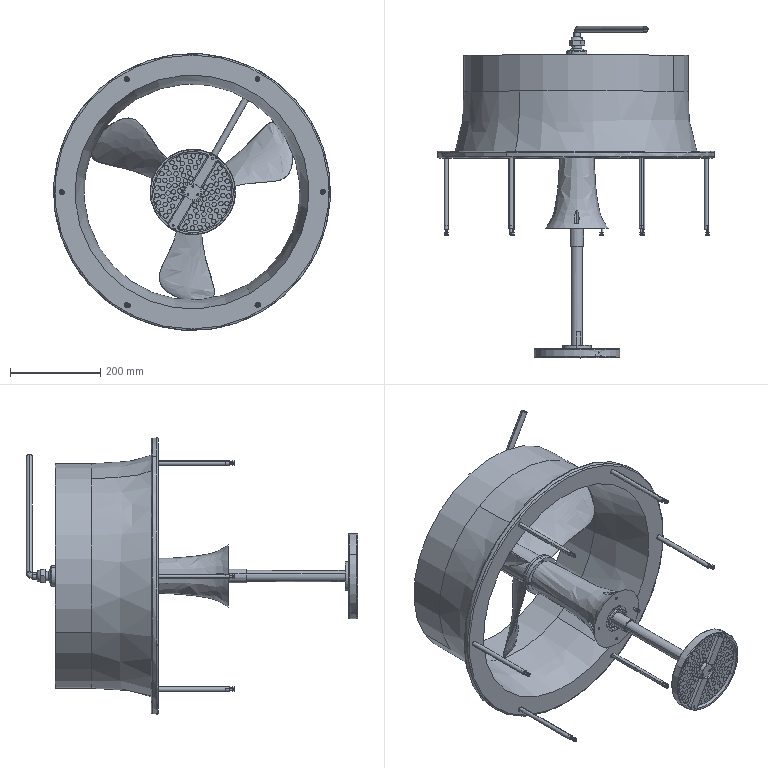Part | NX | features BREP 16 | 27 solids | 1247 faces | box 615 x 737 x 615 mm | volume 7539199 mm3 | cylinder 460 | plane 325 | torus 183 | sphere 128 | cone 80 | spline 71 | commonest cylinder face diameters 10 x201 5 x52 22 x26 16 x18 5.2 x16 8.5 x14